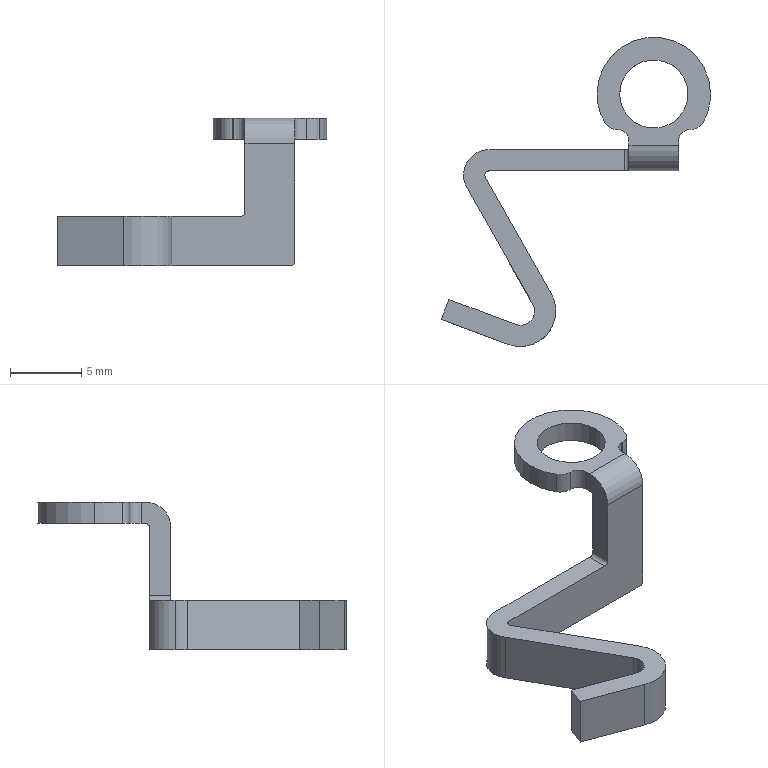Part | STEP file | TQ-DD-1105-THTerminalA1010_デフォルト | 1 solid | 34 faces | box 18.96 x 21.767 x 10.4 mm | volume 259.607 mm3 | cylinder 19 | plane 15 | commonest cylinder face diameters 0.6 x5 2 x3 3.6 x3 8 x3 1.6 x2 4.8 x2
STEP:
#1=CARTESIAN_POINT('',(-11.896,-5.7,-5.4));
#2=VERTEX_POINT('',#1);
#3=CARTESIAN_POINT('',(-11.596,-5.4,-5.4));
#4=VERTEX_POINT('',#3);
#5=CARTESIAN_POINT('',(-11.596,-5.7,-5.4));
#6=DIRECTION('',(0.,0.,-1.));
#7=DIRECTION('',(-1.,0.,0.));
#8=AXIS2_PLACEMENT_3D('',#5,#6,#7);
#9=CIRCLE('',#8,0.3);
#10=EDGE_CURVE('',#2,#4,#9,.T.);
#11=ORIENTED_EDGE('',*,*,#10,.F.);
#12=CARTESIAN_POINT('',(-11.896,-5.7,-8.9));
#13=VERTEX_POINT('',#12);
#14=CARTESIAN_POINT('',(-11.896,-5.7,-7.15));
#15=DIRECTION('',(0.,0.,-1.));
#16=VECTOR('',#15,1000.);
#17=LINE('',#14,#16);
#18=EDGE_CURVE('',#2,#13,#17,.T.);
#19=ORIENTED_EDGE('',*,*,#18,.T.);
#20=CARTESIAN_POINT('',(-11.596,-5.4,-8.9));
#21=VERTEX_POINT('',#20);
#22=CARTESIAN_POINT('',(-11.596,-5.7,-8.9));
#23=DIRECTION('',(0.,0.,1.));
#24=DIRECTION('',(-1.,0.,0.));
#25=AXIS2_PLACEMENT_3D('',#22,#23,#24);
#26=CIRCLE('',#25,0.3);
#27=EDGE_CURVE('',#21,#13,#26,.T.);
#28=ORIENTED_EDGE('',*,*,#27,.F.);
#29=CARTESIAN_POINT('',(-11.596,-5.4,0.));
#30=DIRECTION('',(0.,0.,-1.));
#31=VECTOR('',#30,1000.);
#32=LINE('',#29,#31);
#33=EDGE_CURVE('',#4,#21,#32,.T.);
#34=ORIENTED_EDGE('',*,*,#33,.F.);
#35=EDGE_LOOP('',(#11,#19,#28,#34));
#36=FACE_OUTER_BOUND('',#35,.T.);
#37=CARTESIAN_POINT('',(-11.596,-5.7,-7.15));
#38=DIRECTION('',(0.,0.,-1.));
#39=DIRECTION('',(-1.,0.,0.));
#40=AXIS2_PLACEMENT_3D('',#37,#38,#39);
#41=CYLINDRICAL_SURFACE('',#40,0.3);
#42=ADVANCED_FACE('',(#36),#41,.F.);
#43=CARTESIAN_POINT('',(-13.163,-6.586,-5.4));
#44=VERTEX_POINT('',#43);
#45=CARTESIAN_POINT('',(-13.396,-5.7,-5.4));
#46=VERTEX_POINT('',#45);
#47=CARTESIAN_POINT('',(-11.596,-5.7,-5.4));
#48=DIRECTION('',(0.,0.,-1.));
#49=DIRECTION('',(-1.,0.,0.));
#50=AXIS2_PLACEMENT_3D('',#47,#48,#49);
#51=CIRCLE('',#50,1.8);
#52=EDGE_CURVE('',#44,#46,#51,.T.);
#53=ORIENTED_EDGE('',*,*,#52,.T.);
#54=CARTESIAN_POINT('',(-13.396,-5.7,-8.9));
#55=VERTEX_POINT('',#54);
#56=CARTESIAN_POINT('',(-13.396,-5.7,-7.15));
#57=DIRECTION('',(0.,0.,-1.));
#58=VECTOR('',#57,1000.);
#59=LINE('',#56,#58);
#60=EDGE_CURVE('',#46,#55,#59,.T.);
#61=ORIENTED_EDGE('',*,*,#60,.T.);
#62=CARTESIAN_POINT('',(-13.163,-6.586,-8.9));
#63=VERTEX_POINT('',#62);
#64=CARTESIAN_POINT('',(-11.596,-5.7,-8.9));
#65=DIRECTION('',(0.,0.,-1.));
#66=DIRECTION('',(-1.,0.,0.));
#67=AXIS2_PLACEMENT_3D('',#64,#65,#66);
#68=CIRCLE('',#67,1.8);
#69=EDGE_CURVE('',#63,#55,#68,.T.);
#70=ORIENTED_EDGE('',*,*,#69,.F.);
#71=CARTESIAN_POINT('',(-13.163,-6.586,-7.15));
#72=DIRECTION('',(0.,0.,1.));
#73=VECTOR('',#72,1000.);
#74=LINE('',#71,#73);
#75=EDGE_CURVE('',#63,#44,#74,.T.);
#76=ORIENTED_EDGE('',*,*,#75,.T.);
#77=EDGE_LOOP('',(#53,#61,#70,#76));
#78=FACE_OUTER_BOUND('',#77,.T.);
#79=CARTESIAN_POINT('',(-11.596,-5.7,-7.15));
#80=DIRECTION('',(0.,0.,-1.));
#81=DIRECTION('',(-1.,0.,0.));
#82=AXIS2_PLACEMENT_3D('',#79,#80,#81);
#83=CYLINDRICAL_SURFACE('',#82,1.8);
#84=ADVANCED_FACE('',(#78),#83,.T.);
#85=CARTESIAN_POINT('',(-2.4,0.,0.));
#86=VERTEX_POINT('',#85);
#87=CARTESIAN_POINT('',(2.4,0.,0.));
#88=VERTEX_POINT('',#87);
#89=CARTESIAN_POINT('',(0.,0.,0.));
#90=DIRECTION('',(0.,0.,1.));
#91=DIRECTION('',(1.,0.,0.));
#92=AXIS2_PLACEMENT_3D('',#89,#90,#91);
#93=CIRCLE('',#92,2.4);
#94=EDGE_CURVE('',#86,#88,#93,.T.);
#95=ORIENTED_EDGE('',*,*,#94,.F.);
#96=CARTESIAN_POINT('',(-2.4,0.,1.5));
#97=VERTEX_POINT('',#96);
#98=CARTESIAN_POINT('',(-2.4,0.,0.75));
#99=DIRECTION('',(0.,0.,1.));
#100=VECTOR('',#99,1000.);
#101=LINE('',#98,#100);
#102=EDGE_CURVE('',#86,#97,#101,.T.);
#103=ORIENTED_EDGE('',*,*,#102,.T.);
#104=CARTESIAN_POINT('',(2.4,0.,1.5));
#105=VERTEX_POINT('',#104);
#106=CARTESIAN_POINT('',(0.,0.,1.5));
#107=DIRECTION('',(0.,0.,-1.));
#108=DIRECTION('',(1.,0.,0.));
#109=AXIS2_PLACEMENT_3D('',#106,#107,#108);
#110=CIRCLE('',#109,2.4);
#111=EDGE_CURVE('',#105,#97,#110,.T.);
#112=ORIENTED_EDGE('',*,*,#111,.F.);
#113=CARTESIAN_POINT('',(2.4,0.,0.75));
#114=DIRECTION('',(0.,0.,1.));
#115=VECTOR('',#114,1000.);
#116=LINE('',#113,#115);
#117=EDGE_CURVE('',#88,#105,#116,.T.);
#118=ORIENTED_EDGE('',*,*,#117,.F.);
#119=EDGE_LOOP('',(#95,#103,#112,#118));
#120=FACE_OUTER_BOUND('',#119,.T.);
#121=CARTESIAN_POINT('',(0.,0.,0.75));
#122=DIRECTION('',(0.,0.,1.));
#123=DIRECTION('',(1.,0.,0.));
#124=AXIS2_PLACEMENT_3D('',#121,#122,#123);
#125=CYLINDRICAL_SURFACE('',#124,2.4);
#126=ADVANCED_FACE('',(#120),#125,.F.);
#127=CARTESIAN_POINT('',(4.,0.,0.));
#128=VERTEX_POINT('',#127);
#129=CARTESIAN_POINT('',(-4.,0.,0.));
#130=VERTEX_POINT('',#129);
#131=CARTESIAN_POINT('',(0.,0.,0.));
#132=DIRECTION('',(0.,0.,1.));
#133=DIRECTION('',(1.,0.,0.));
#134=AXIS2_PLACEMENT_3D('',#131,#132,#133);
#135=CIRCLE('',#134,4.);
#136=EDGE_CURVE('',#128,#130,#135,.T.);
#137=ORIENTED_EDGE('',*,*,#136,.T.);
#138=CARTESIAN_POINT('',(-4.,0.,1.5));
#139=VERTEX_POINT('',#138);
#140=CARTESIAN_POINT('',(-4.,0.,0.75));
#141=DIRECTION('',(0.,0.,1.));
#142=VECTOR('',#141,1000.);
#143=LINE('',#140,#142);
#144=EDGE_CURVE('',#130,#139,#143,.T.);
#145=ORIENTED_EDGE('',*,*,#144,.T.);
#146=CARTESIAN_POINT('',(4.,0.,1.5));
#147=VERTEX_POINT('',#146);
#148=CARTESIAN_POINT('',(0.,0.,1.5));
#149=DIRECTION('',(0.,0.,1.));
#150=DIRECTION('',(1.,0.,0.));
#151=AXIS2_PLACEMENT_3D('',#148,#149,#150);
#152=CIRCLE('',#151,4.);
#153=EDGE_CURVE('',#147,#139,#152,.T.);
#154=ORIENTED_EDGE('',*,*,#153,.F.);
#155=CARTESIAN_POINT('',(4.,0.,0.75));
#156=DIRECTION('',(0.,0.,1.));
#157=VECTOR('',#156,1000.);
#158=LINE('',#155,#157);
#159=EDGE_CURVE('',#128,#147,#158,.T.);
#160=ORIENTED_EDGE('',*,*,#159,.F.);
#161=EDGE_LOOP('',(#137,#145,#154,#160));
#162=FACE_OUTER_BOUND('',#161,.T.);
#163=CARTESIAN_POINT('',(0.,0.,0.75));
#164=DIRECTION('',(0.,0.,1.));
#165=DIRECTION('',(1.,0.,0.));
#166=AXIS2_PLACEMENT_3D('',#163,#164,#165);
#167=CYLINDRICAL_SURFACE('',#166,4.);
#168=ADVANCED_FACE('',(#162),#167,.T.);
#169=CARTESIAN_POINT('',(3.464,-2.,0.));
#170=VERTEX_POINT('',#169);
#171=CARTESIAN_POINT('',(0.,0.,0.));
#172=DIRECTION('',(0.,0.,1.));
#173=DIRECTION('',(1.,0.,0.));
#174=AXIS2_PLACEMENT_3D('',#171,#172,#173);
#175=CIRCLE('',#174,4.);
#176=EDGE_CURVE('',#170,#128,#175,.T.);
#177=ORIENTED_EDGE('',*,*,#176,.T.);
#178=ORIENTED_EDGE('',*,*,#159,.T.);
#179=CARTESIAN_POINT('',(3.464,-2.,1.5));
#180=VERTEX_POINT('',#179);
#181=CARTESIAN_POINT('',(0.,0.,1.5));
#182=DIRECTION('',(0.,0.,1.));
#183=DIRECTION('',(1.,0.,0.));
#184=AXIS2_PLACEMENT_3D('',#181,#182,#183);
#185=CIRCLE('',#184,4.);
#186=EDGE_CURVE('',#180,#147,#185,.T.);
#187=ORIENTED_EDGE('',*,*,#186,.F.);
#188=CARTESIAN_POINT('',(3.464,-2.,0.75));
#189=DIRECTION('',(0.,0.,1.));
#190=VECTOR('',#189,1000.);
#191=LINE('',#188,#190);
#192=EDGE_CURVE('',#170,#180,#191,.T.);
#193=ORIENTED_EDGE('',*,*,#192,.F.);
#194=EDGE_LOOP('',(#177,#178,#187,#193));
#195=FACE_OUTER_BOUND('',#194,.T.);
#196=CARTESIAN_POINT('',(0.,0.,0.75));
#197=DIRECTION('',(0.,0.,1.));
#198=DIRECTION('',(1.,0.,0.));
#199=AXIS2_PLACEMENT_3D('',#196,#197,#198);
#200=CYLINDRICAL_SURFACE('',#199,4.);
#201=ADVANCED_FACE('',(#195),#200,.T.);
#202=CARTESIAN_POINT('',(1.75,-5.4,-0.3));
#203=VERTEX_POINT('',#202);
#204=CARTESIAN_POINT('',(-1.75,-5.4,-0.3));
#205=VERTEX_POINT('',#204);
#206=CARTESIAN_POINT('',(-1.75,-5.4,-0.3));
#207=DIRECTION('',(-1.,0.,0.));
#208=VECTOR('',#207,1000.);
#209=LINE('',#206,#208);
#210=EDGE_CURVE('',#203,#205,#209,.T.);
#211=ORIENTED_EDGE('',*,*,#210,.T.);
#212=CARTESIAN_POINT('',(-1.75,-5.4,-5.1));
#213=VERTEX_POINT('',#212);
#214=CARTESIAN_POINT('',(-1.75,-5.4,0.));
#215=DIRECTION('',(0.,0.,-1.));
#216=VECTOR('',#215,1000.);
#217=LINE('',#214,#216);
#218=EDGE_CURVE('',#205,#213,#217,.T.);
#219=ORIENTED_EDGE('',*,*,#218,.T.);
#220=CARTESIAN_POINT('',(-2.05,-5.4,-5.4));
#221=VERTEX_POINT('',#220);
#222=CARTESIAN_POINT('',(-2.05,-5.4,-5.1));
#223=DIRECTION('',(0.,1.,0.));
#224=DIRECTION('',(0.,0.,1.));
#225=AXIS2_PLACEMENT_3D('',#222,#223,#224);
#226=CIRCLE('',#225,0.3);
#227=EDGE_CURVE('',#213,#221,#226,.T.);
#228=ORIENTED_EDGE('',*,*,#227,.T.);
#229=CARTESIAN_POINT('',(-1.75,-5.4,-5.4));
#230=DIRECTION('',(-1.,0.,0.));
#231=VECTOR('',#230,1000.);
#232=LINE('',#229,#231);
#233=EDGE_CURVE('',#221,#4,#232,.T.);
#234=ORIENTED_EDGE('',*,*,#233,.T.);
#235=ORIENTED_EDGE('',*,*,#33,.T.);
#236=CARTESIAN_POINT('',(1.45,-5.4,-8.9));
#237=VERTEX_POINT('',#236);
#238=CARTESIAN_POINT('',(-1.75,-5.4,-8.9));
#239=DIRECTION('',(1.,0.,0.));
#240=VECTOR('',#239,1000.);
#241=LINE('',#238,#240);
#242=EDGE_CURVE('',#21,#237,#241,.T.);
#243=ORIENTED_EDGE('',*,*,#242,.T.);
#244=CARTESIAN_POINT('',(1.75,-5.4,-8.6));
#245=VERTEX_POINT('',#244);
#246=CARTESIAN_POINT('',(1.45,-5.4,-8.6));
#247=DIRECTION('',(0.,1.,0.));
#248=DIRECTION('',(0.,0.,1.));
#249=AXIS2_PLACEMENT_3D('',#246,#247,#248);
#250=CIRCLE('',#249,0.3);
#251=EDGE_CURVE('',#245,#237,#250,.T.);
#252=ORIENTED_EDGE('',*,*,#251,.F.);
#253=CARTESIAN_POINT('',(1.75,-5.4,0.));
#254=DIRECTION('',(0.,0.,1.));
#255=VECTOR('',#254,1000.);
#256=LINE('',#253,#255);
#257=EDGE_CURVE('',#245,#203,#256,.T.);
#258=ORIENTED_EDGE('',*,*,#257,.T.);
#259=EDGE_LOOP('',(#211,#219,#228,#234,#235,#243,#252,#258));
#260=FACE_OUTER_BOUND('',#259,.T.);
#261=CARTESIAN_POINT('',(-1.75,-5.4,0.));
#262=DIRECTION('',(0.,-1.,0.));
#263=DIRECTION('',(0.,0.,-1.));
#264=AXIS2_PLACEMENT_3D('',#261,#262,#263);
#265=PLANE('',#264);
#266=ADVANCED_FACE('',(#260),#265,.T.);
#267=CARTESIAN_POINT('',(-1.75,-3.9,-0.3));
#268=VERTEX_POINT('',#267);
#269=CARTESIAN_POINT('',(-1.75,-3.9,-5.1));
#270=VERTEX_POINT('',#269);
#271=CARTESIAN_POINT('',(-1.75,-3.9,0.));
#272=DIRECTION('',(0.,0.,-1.));
#273=VECTOR('',#272,1000.);
#274=LINE('',#271,#273);
#275=EDGE_CURVE('',#268,#270,#274,.T.);
#276=ORIENTED_EDGE('',*,*,#275,.T.);
#277=CARTESIAN_POINT('',(-1.75,-2.5,-5.1));
#278=DIRECTION('',(0.,-1.,0.));
#279=VECTOR('',#278,1000.);
#280=LINE('',#277,#279);
#281=EDGE_CURVE('',#270,#213,#280,.T.);
#282=ORIENTED_EDGE('',*,*,#281,.T.);
#283=ORIENTED_EDGE('',*,*,#218,.F.);
#284=CARTESIAN_POINT('',(-1.75,-3.6,1.5));
#285=VERTEX_POINT('',#284);
#286=CARTESIAN_POINT('',(-1.75,-3.6,-0.3));
#287=DIRECTION('',(-1.,0.,0.));
#288=DIRECTION('',(0.,0.,-1.));
#289=AXIS2_PLACEMENT_3D('',#286,#287,#288);
#290=CIRCLE('',#289,1.8);
#291=EDGE_CURVE('',#205,#285,#290,.T.);
#292=ORIENTED_EDGE('',*,*,#291,.T.);
#293=CARTESIAN_POINT('',(-1.75,-3.3,1.5));
#294=VERTEX_POINT('',#293);
#295=CARTESIAN_POINT('',(-1.75,0.,1.5));
#296=DIRECTION('',(0.,-1.,0.));
#297=VECTOR('',#296,1000.);
#298=LINE('',#295,#297);
#299=EDGE_CURVE('',#294,#285,#298,.T.);
#300=ORIENTED_EDGE('',*,*,#299,.F.);
#301=CARTESIAN_POINT('',(-1.75,-3.3,0.));
#302=VERTEX_POINT('',#301);
#303=CARTESIAN_POINT('',(-1.75,-3.3,0.));
#304=DIRECTION('',(0.,0.,-1.));
#305=VECTOR('',#304,1000.);
#306=LINE('',#303,#305);
#307=EDGE_CURVE('',#294,#302,#306,.T.);
#308=ORIENTED_EDGE('',*,*,#307,.T.);
#309=CARTESIAN_POINT('',(-1.75,-3.6,0.));
#310=VERTEX_POINT('',#309);
#311=CARTESIAN_POINT('',(-1.75,0.,0.));
#312=DIRECTION('',(0.,-1.,0.));
#313=VECTOR('',#312,1000.);
#314=LINE('',#311,#313);
#315=EDGE_CURVE('',#302,#310,#314,.T.);
#316=ORIENTED_EDGE('',*,*,#315,.T.);
#317=CARTESIAN_POINT('',(-1.75,-3.6,-0.3));
#318=DIRECTION('',(1.,0.,0.));
#319=DIRECTION('',(0.,0.,1.));
#320=AXIS2_PLACEMENT_3D('',#317,#318,#319);
#321=CIRCLE('',#320,0.3);
#322=EDGE_CURVE('',#310,#268,#321,.T.);
#323=ORIENTED_EDGE('',*,*,#322,.T.);
#324=EDGE_LOOP('',(#276,#282,#283,#292,#300,#308,#316,#323));
#325=FACE_OUTER_BOUND('',#324,.T.);
#326=CARTESIAN_POINT('',(-1.75,-2.5,0.));
#327=DIRECTION('',(-1.,0.,0.));
#328=DIRECTION('',(0.,0.,1.));
#329=AXIS2_PLACEMENT_3D('',#326,#327,#328);
#330=PLANE('',#329);
#331=ADVANCED_FACE('',(#325),#330,.T.);
#332=ORIENTED_EDGE('',*,*,#291,.F.);
#333=ORIENTED_EDGE('',*,*,#210,.F.);
#334=CARTESIAN_POINT('',(1.75,-3.6,1.5));
#335=VERTEX_POINT('',#334);
#336=CARTESIAN_POINT('',(1.75,-3.6,-0.3));
#337=DIRECTION('',(-1.,0.,0.));
#338=DIRECTION('',(0.,0.,-1.));
#339=AXIS2_PLACEMENT_3D('',#336,#337,#338);
#340=CIRCLE('',#339,1.8);
#341=EDGE_CURVE('',#203,#335,#340,.T.);
#342=ORIENTED_EDGE('',*,*,#341,.T.);
#343=CARTESIAN_POINT('',(0.,-3.6,1.5));
#344=DIRECTION('',(-1.,0.,0.));
#345=VECTOR('',#344,1000.);
#346=LINE('',#343,#345);
#347=EDGE_CURVE('',#335,#285,#346,.T.);
#348=ORIENTED_EDGE('',*,*,#347,.T.);
#349=EDGE_LOOP('',(#332,#333,#342,#348));
#350=FACE_OUTER_BOUND('',#349,.T.);
#351=CARTESIAN_POINT('',(0.,-3.6,-0.3));
#352=DIRECTION('',(1.,0.,0.));
#353=DIRECTION('',(0.,0.,-1.));
#354=AXIS2_PLACEMENT_3D('',#351,#352,#353);
#355=CYLINDRICAL_SURFACE('',#354,1.8);
#356=ADVANCED_FACE('',(#350),#355,.T.);
#357=ORIENTED_EDGE('',*,*,#257,.F.);
#358=CARTESIAN_POINT('',(1.75,-3.9,-8.6));
#359=VERTEX_POINT('',#358);
#360=CARTESIAN_POINT('',(1.75,-5.4,-8.6));
#361=DIRECTION('',(0.,1.,0.));
#362=VECTOR('',#361,1000.);
#363=LINE('',#360,#362);
#364=EDGE_CURVE('',#245,#359,#363,.T.);
#365=ORIENTED_EDGE('',*,*,#364,.T.);
#366=CARTESIAN_POINT('',(1.75,-3.9,-0.3));
#367=VERTEX_POINT('',#366);
#368=CARTESIAN_POINT('',(1.75,-3.9,0.));
#369=DIRECTION('',(0.,0.,1.));
#370=VECTOR('',#369,1000.);
#371=LINE('',#368,#370);
#372=EDGE_CURVE('',#359,#367,#371,.T.);
#373=ORIENTED_EDGE('',*,*,#372,.T.);
#374=CARTESIAN_POINT('',(1.75,-3.6,0.));
#375=VERTEX_POINT('',#374);
#376=CARTESIAN_POINT('',(1.75,-3.6,-0.3));
#377=DIRECTION('',(-1.,0.,0.));
#378=DIRECTION('',(0.,0.,1.));
#379=AXIS2_PLACEMENT_3D('',#376,#377,#378);
#380=CIRCLE('',#379,0.3);
#381=EDGE_CURVE('',#367,#375,#380,.T.);
#382=ORIENTED_EDGE('',*,*,#381,.T.);
#383=CARTESIAN_POINT('',(1.75,-3.3,0.));
#384=VERTEX_POINT('',#383);
#385=CARTESIAN_POINT('',(1.75,0.,0.));
#386=DIRECTION('',(0.,1.,0.));
#387=VECTOR('',#386,1000.);
#388=LINE('',#385,#387);
#389=EDGE_CURVE('',#375,#384,#388,.T.);
#390=ORIENTED_EDGE('',*,*,#389,.T.);
#391=CARTESIAN_POINT('',(1.75,-3.3,1.5));
#392=VERTEX_POINT('',#391);
#393=CARTESIAN_POINT('',(1.75,-3.3,0.));
#394=DIRECTION('',(0.,0.,1.));
#395=VECTOR('',#394,1000.);
#396=LINE('',#393,#395);
#397=EDGE_CURVE('',#384,#392,#396,.T.);
#398=ORIENTED_EDGE('',*,*,#397,.T.);
#399=CARTESIAN_POINT('',(1.75,-5.4,1.5));
#400=DIRECTION('',(0.,-1.,0.));
#401=VECTOR('',#400,1000.);
#402=LINE('',#399,#401);
#403=EDGE_CURVE('',#392,#335,#402,.T.);
#404=ORIENTED_EDGE('',*,*,#403,.T.);
#405=ORIENTED_EDGE('',*,*,#341,.F.);
#406=EDGE_LOOP('',(#357,#365,#373,#382,#390,#398,#404,#405));
#407=FACE_OUTER_BOUND('',#406,.T.);
#408=CARTESIAN_POINT('',(1.75,-5.4,0.));
#409=DIRECTION('',(1.,0.,0.));
#410=DIRECTION('',(0.,0.,-1.));
#411=AXIS2_PLACEMENT_3D('',#408,#409,#410);
#412=PLANE('',#411);
#413=ADVANCED_FACE('',(#407),#412,.T.);
#414=CARTESIAN_POINT('',(-11.596,-3.9,-8.9));
#415=VERTEX_POINT('',#414);
#416=CARTESIAN_POINT('',(1.45,-3.9,-8.9));
#417=VERTEX_POINT('',#416);
#418=CARTESIAN_POINT('',(0.,-3.9,-8.9));
#419=DIRECTION('',(1.,0.,0.));
#420=VECTOR('',#419,1000.);
#421=LINE('',#418,#420);
#422=EDGE_CURVE('',#415,#417,#421,.T.);
#423=ORIENTED_EDGE('',*,*,#422,.T.);
#424=CARTESIAN_POINT('',(1.45,-5.4,-8.9));
#425=DIRECTION('',(0.,-1.,0.));
#426=VECTOR('',#425,1000.);
#427=LINE('',#424,#426);
#428=EDGE_CURVE('',#417,#237,#427,.T.);
#429=ORIENTED_EDGE('',*,*,#428,.T.);
#430=ORIENTED_EDGE('',*,*,#242,.F.);
#431=ORIENTED_EDGE('',*,*,#27,.T.);
#432=CARTESIAN_POINT('',(-11.857,-5.848,-8.9));
#433=VERTEX_POINT('',#432);
#434=CARTESIAN_POINT('',(-11.596,-5.7,-8.9));
#435=DIRECTION('',(0.,0.,1.));
#436=DIRECTION('',(-1.,0.,0.));
#437=AXIS2_PLACEMENT_3D('',#434,#435,#436);
#438=CIRCLE('',#437,0.3);
#439=EDGE_CURVE('',#13,#433,#438,.T.);
#440=ORIENTED_EDGE('',*,*,#439,.T.);
#441=CARTESIAN_POINT('',(-7.225,-14.036,-8.9));
#442=VERTEX_POINT('',#441);
#443=CARTESIAN_POINT('',(-11.857,-5.848,-8.9));
#444=DIRECTION('',(0.4924,-0.8704,0.));
#445=VECTOR('',#444,1000.);
#446=LINE('',#443,#445);
#447=EDGE_CURVE('',#433,#442,#446,.T.);
#448=ORIENTED_EDGE('',*,*,#447,.T.);
#449=CARTESIAN_POINT('',(-10.276,-17.608,-8.9));
#450=VERTEX_POINT('',#449);
#451=CARTESIAN_POINT('',(-9.401,-15.267,-8.9));
#452=DIRECTION('',(0.,0.,-1.));
#453=DIRECTION('',(-1.,0.,0.));
#454=AXIS2_PLACEMENT_3D('',#451,#452,#453);
#455=CIRCLE('',#454,2.5);
#456=EDGE_CURVE('',#442,#450,#455,.T.);
#457=ORIENTED_EDGE('',*,*,#456,.T.);
#458=CARTESIAN_POINT('',(-14.96,-15.857,-8.9));
#459=VERTEX_POINT('',#458);
#460=CARTESIAN_POINT('',(-10.276,-17.608,-8.9));
#461=DIRECTION('',(-0.9367,0.3502,0.));
#462=VECTOR('',#461,1000.);
#463=LINE('',#460,#462);
#464=EDGE_CURVE('',#450,#459,#463,.T.);
#465=ORIENTED_EDGE('',*,*,#464,.T.);
#466=CARTESIAN_POINT('',(-14.434,-14.452,-8.9));
#467=VERTEX_POINT('',#466);
#468=CARTESIAN_POINT('',(-14.434,-14.452,-8.9));
#469=DIRECTION('',(-0.3502,-0.9367,0.));
#470=VECTOR('',#469,1000.);
#471=LINE('',#468,#470);
#472=EDGE_CURVE('',#467,#459,#471,.T.);
#473=ORIENTED_EDGE('',*,*,#472,.F.);
#474=CARTESIAN_POINT('',(-9.751,-16.203,-8.9));
#475=VERTEX_POINT('',#474);
#476=CARTESIAN_POINT('',(-14.434,-14.452,-8.9));
#477=DIRECTION('',(0.9367,-0.3502,0.));
#478=VECTOR('',#477,1000.);
#479=LINE('',#476,#478);
#480=EDGE_CURVE('',#467,#475,#479,.T.);
#481=ORIENTED_EDGE('',*,*,#480,.T.);
#482=CARTESIAN_POINT('',(-8.53,-14.774,-8.9));
#483=VERTEX_POINT('',#482);
#484=CARTESIAN_POINT('',(-9.401,-15.267,-8.9));
#485=DIRECTION('',(0.,0.,1.));
#486=DIRECTION('',(-1.,0.,0.));
#487=AXIS2_PLACEMENT_3D('',#484,#485,#486);
#488=CIRCLE('',#487,1.);
#489=EDGE_CURVE('',#475,#483,#488,.T.);
#490=ORIENTED_EDGE('',*,*,#489,.T.);
#491=CARTESIAN_POINT('',(-8.53,-14.774,-8.9));
#492=DIRECTION('',(-0.4924,0.8704,0.));
#493=VECTOR('',#492,1000.);
#494=LINE('',#491,#493);
#495=EDGE_CURVE('',#483,#63,#494,.T.);
#496=ORIENTED_EDGE('',*,*,#495,.T.);
#497=ORIENTED_EDGE('',*,*,#69,.T.);
#498=CARTESIAN_POINT('',(-11.596,-5.7,-8.9));
#499=DIRECTION('',(0.,0.,-1.));
#500=DIRECTION('',(-1.,0.,0.));
#501=AXIS2_PLACEMENT_3D('',#498,#499,#500);
#502=CIRCLE('',#501,1.8);
#503=EDGE_CURVE('',#55,#415,#502,.T.);
#504=ORIENTED_EDGE('',*,*,#503,.T.);
#505=EDGE_LOOP('',(#423,#429,#430,#431,#440,#448,#457,#465,#473,#481,#490,#496,#497,#504));
#506=FACE_OUTER_BOUND('',#505,.T.);
#507=CARTESIAN_POINT('',(0.,-5.4,-8.9));
#508=DIRECTION('',(0.,0.,-1.));
#509=DIRECTION('',(-1.,0.,0.));
#510=AXIS2_PLACEMENT_3D('',#507,#508,#509);
#511=PLANE('',#510);
#512=ADVANCED_FACE('',(#506),#511,.T.);
#513=ORIENTED_EDGE('',*,*,#18,.F.);
#514=CARTESIAN_POINT('',(-11.857,-5.848,-5.4));
#515=VERTEX_POINT('',#514);
#516=CARTESIAN_POINT('',(-11.596,-5.7,-5.4));
#517=DIRECTION('',(0.,0.,-1.));
#518=DIRECTION('',(-1.,0.,0.));
#519=AXIS2_PLACEMENT_3D('',#516,#517,#518);
#520=CIRCLE('',#519,0.3);
#521=EDGE_CURVE('',#515,#2,#520,.T.);
#522=ORIENTED_EDGE('',*,*,#521,.F.);
#523=CARTESIAN_POINT('',(-11.857,-5.848,-7.15));
#524=DIRECTION('',(0.,0.,1.));
#525=VECTOR('',#524,1000.);
#526=LINE('',#523,#525);
#527=EDGE_CURVE('',#433,#515,#526,.T.);
#528=ORIENTED_EDGE('',*,*,#527,.F.);
#529=ORIENTED_EDGE('',*,*,#439,.F.);
#530=EDGE_LOOP('',(#513,#522,#528,#529));
#531=FACE_OUTER_BOUND('',#530,.T.);
#532=CARTESIAN_POINT('',(-11.596,-5.7,-7.15));
#533=DIRECTION('',(0.,0.,-1.));
#534=DIRECTION('',(-1.,0.,0.));
#535=AXIS2_PLACEMENT_3D('',#532,#533,#534);
#536=CYLINDRICAL_SURFACE('',#535,0.3);
#537=ADVANCED_FACE('',(#531),#536,.F.);
#538=CARTESIAN_POINT('',(-11.596,-3.9,-5.4));
#539=VERTEX_POINT('',#538);
#540=CARTESIAN_POINT('',(-2.05,-3.9,-5.4));
#541=VERTEX_POINT('',#540);
#542=CARTESIAN_POINT('',(0.,-3.9,-5.4));
#543=DIRECTION('',(1.,0.,0.));
#544=VECTOR('',#543,1000.);
#545=LINE('',#542,#544);
#546=EDGE_CURVE('',#539,#541,#545,.T.);
#547=ORIENTED_EDGE('',*,*,#546,.F.);
#548=CARTESIAN_POINT('',(-11.596,-5.7,-5.4));
#549=DIRECTION('',(0.,0.,-1.));
#550=DIRECTION('',(-1.,0.,0.));
#551=AXIS2_PLACEMENT_3D('',#548,#549,#550);
#552=CIRCLE('',#551,1.8);
#553=EDGE_CURVE('',#46,#539,#552,.T.);
#554=ORIENTED_EDGE('',*,*,#553,.F.);
#555=ORIENTED_EDGE('',*,*,#52,.F.);
#556=CARTESIAN_POINT('',(-8.53,-14.774,-5.4));
#557=VERTEX_POINT('',#556);
#558=CARTESIAN_POINT('',(-8.53,-14.774,-5.4));
#559=DIRECTION('',(-0.4924,0.8704,0.));
#560=VECTOR('',#559,1000.);
#561=LINE('',#558,#560);
#562=EDGE_CURVE('',#557,#44,#561,.T.);
#563=ORIENTED_EDGE('',*,*,#562,.F.);
#564=CARTESIAN_POINT('',(-9.751,-16.203,-5.4));
#565=VERTEX_POINT('',#564);
#566=CARTESIAN_POINT('',(-9.401,-15.267,-5.4));
#567=DIRECTION('',(0.,0.,1.));
#568=DIRECTION('',(-1.,0.,0.));
#569=AXIS2_PLACEMENT_3D('',#566,#567,#568);
#570=CIRCLE('',#569,1.);
#571=EDGE_CURVE('',#565,#557,#570,.T.);
#572=ORIENTED_EDGE('',*,*,#571,.F.);
#573=CARTESIAN_POINT('',(-14.434,-14.452,-5.4));
#574=VERTEX_POINT('',#573);
#575=CARTESIAN_POINT('',(-14.434,-14.452,-5.4));
#576=DIRECTION('',(0.9367,-0.3502,0.));
#577=VECTOR('',#576,1000.);
#578=LINE('',#575,#577);
#579=EDGE_CURVE('',#574,#565,#578,.T.);
#580=ORIENTED_EDGE('',*,*,#579,.F.);
#581=CARTESIAN_POINT('',(-14.96,-15.857,-5.4));
#582=VERTEX_POINT('',#581);
#583=CARTESIAN_POINT('',(-14.434,-14.452,-5.4));
#584=DIRECTION('',(0.3502,0.9367,0.));
#585=VECTOR('',#584,1000.);
#586=LINE('',#583,#585);
#587=EDGE_CURVE('',#582,#574,#586,.T.);
#588=ORIENTED_EDGE('',*,*,#587,.F.);
#589=CARTESIAN_POINT('',(-10.276,-17.608,-5.4));
#590=VERTEX_POINT('',#589);
#591=CARTESIAN_POINT('',(-10.276,-17.608,-5.4));
#592=DIRECTION('',(-0.9367,0.3502,0.));
#593=VECTOR('',#592,1000.);
#594=LINE('',#591,#593);
#595=EDGE_CURVE('',#590,#582,#594,.T.);
#596=ORIENTED_EDGE('',*,*,#595,.F.);
#597=CARTESIAN_POINT('',(-7.225,-14.036,-5.4));
#598=VERTEX_POINT('',#597);
#599=CARTESIAN_POINT('',(-9.401,-15.267,-5.4));
#600=DIRECTION('',(0.,0.,-1.));
#601=DIRECTION('',(-1.,0.,0.));
#602=AXIS2_PLACEMENT_3D('',#599,#600,#601);
#603=CIRCLE('',#602,2.5);
#604=EDGE_CURVE('',#598,#590,#603,.T.);
#605=ORIENTED_EDGE('',*,*,#604,.F.);
#606=CARTESIAN_POINT('',(-11.857,-5.848,-5.4));
#607=DIRECTION('',(0.4924,-0.8704,0.));
#608=VECTOR('',#607,1000.);
#609=LINE('',#606,#608);
#610=EDGE_CURVE('',#515,#598,#609,.T.);
#611=ORIENTED_EDGE('',*,*,#610,.F.);
#612=ORIENTED_EDGE('',*,*,#521,.T.);
#613=ORIENTED_EDGE('',*,*,#10,.T.);
#614=ORIENTED_EDGE('',*,*,#233,.F.);
#615=CARTESIAN_POINT('',(-2.05,0.,-5.4));
#616=DIRECTION('',(0.,-1.,0.));
#617=VECTOR('',#616,1000.);
#618=LINE('',#615,#617);
#619=EDGE_CURVE('',#541,#221,#618,.T.);
#620=ORIENTED_EDGE('',*,*,#619,.F.);
#621=EDGE_LOOP('',(#547,#554,#555,#563,#572,#580,#588,#596,#605,#611,#612,#613,#614,#620));
#622=FACE_OUTER_BOUND('',#621,.T.);
#623=CARTESIAN_POINT('',(0.,0.,-5.4));
#624=DIRECTION('',(0.,0.,-1.));
#625=DIRECTION('',(-1.,0.,0.));
#626=AXIS2_PLACEMENT_3D('',#623,#624,#625);
#627=PLANE('',#626);
#628=ADVANCED_FACE('',(#622),#627,.F.);
#629=CARTESIAN_POINT('',(-2.05,-3.9,-5.1));
#630=DIRECTION('',(0.,-1.,0.));
#631=DIRECTION('',(0.,0.,1.));
#632=AXIS2_PLACEMENT_3D('',#629,#630,#631);
#633=CIRCLE('',#632,0.3);
#634=EDGE_CURVE('',#541,#270,#633,.T.);
#635=ORIENTED_EDGE('',*,*,#634,.F.);
#636=ORIENTED_EDGE('',*,*,#619,.T.);
#637=ORIENTED_EDGE('',*,*,#227,.F.);
#638=ORIENTED_EDGE('',*,*,#281,.F.);
#639=EDGE_LOOP('',(#635,#636,#637,#638));
#640=FACE_OUTER_BOUND('',#639,.T.);
#641=CARTESIAN_POINT('',(-2.05,-10.833,-5.1));
#642=DIRECTION('',(0.,1.,0.));
#643=DIRECTION('',(0.,0.,1.));
#644=AXIS2_PLACEMENT_3D('',#641,#642,#643);
#645=CYLINDRICAL_SURFACE('',#644,0.3);
#646=ADVANCED_FACE('',(#640),#645,.F.);
#647=CARTESIAN_POINT('',(0.,-3.9,-0.3));
#648=DIRECTION('',(-1.,0.,0.));
#649=VECTOR('',#648,1000.);
#650=LINE('',#647,#649);
#651=EDGE_CURVE('',#367,#268,#650,.T.);
#652=ORIENTED_EDGE('',*,*,#651,.F.);
#653=ORIENTED_EDGE('',*,*,#372,.F.);
#654=CARTESIAN_POINT('',(1.45,-3.9,-8.6));
#655=DIRECTION('',(0.,-1.,0.));
#656=DIRECTION('',(0.,0.,1.));
#657=AXIS2_PLACEMENT_3D('',#654,#655,#656);
#658=CIRCLE('',#657,0.3);
#659=EDGE_CURVE('',#417,#359,#658,.T.);
#660=ORIENTED_EDGE('',*,*,#659,.F.);
#661=ORIENTED_EDGE('',*,*,#422,.F.);
#662=CARTESIAN_POINT('',(-11.596,-3.9,1.5));
#663=DIRECTION('',(0.,0.,-1.));
#664=VECTOR('',#663,1000.);
#665=LINE('',#662,#664);
#666=EDGE_CURVE('',#539,#415,#665,.T.);
#667=ORIENTED_EDGE('',*,*,#666,.F.);
#668=ORIENTED_EDGE('',*,*,#546,.T.);
#669=ORIENTED_EDGE('',*,*,#634,.T.);
#670=ORIENTED_EDGE('',*,*,#275,.F.);
#671=EDGE_LOOP('',(#652,#653,#660,#661,#667,#668,#669,#670));
#672=FACE_OUTER_BOUND('',#671,.T.);
#673=CARTESIAN_POINT('',(0.,-3.9,1.5));
#674=DIRECTION('',(0.,-1.,0.));
#675=DIRECTION('',(0.,0.,-1.));
#676=AXIS2_PLACEMENT_3D('',#673,#674,#675);
#677=PLANE('',#676);
#678=ADVANCED_FACE('',(#672),#677,.F.);
#679=CARTESIAN_POINT('',(-2.55,-2.5,1.5));
#680=VERTEX_POINT('',#679);
#681=CARTESIAN_POINT('',(-2.55,-3.3,1.5));
#682=DIRECTION('',(0.,0.,-1.));
#683=DIRECTION('',(1.,0.,0.));
#684=AXIS2_PLACEMENT_3D('',#681,#682,#683);
#685=CIRCLE('',#684,0.8);
#686=EDGE_CURVE('',#680,#294,#685,.T.);
#687=ORIENTED_EDGE('',*,*,#686,.F.);
#688=CARTESIAN_POINT('',(-2.55,-2.5,0.));
#689=VERTEX_POINT('',#688);
#690=CARTESIAN_POINT('',(-2.55,-2.5,-3.7));
#691=DIRECTION('',(0.,0.,1.));
#692=VECTOR('',#691,1000.);
#693=LINE('',#690,#692);
#694=EDGE_CURVE('',#689,#680,#693,.T.);
#695=ORIENTED_EDGE('',*,*,#694,.F.);
#696=CARTESIAN_POINT('',(-2.55,-3.3,0.));
#697=DIRECTION('',(0.,0.,-1.));
#698=DIRECTION('',(1.,0.,0.));
#699=AXIS2_PLACEMENT_3D('',#696,#697,#698);
#700=CIRCLE('',#699,0.8);
#701=EDGE_CURVE('',#689,#302,#700,.T.);
#702=ORIENTED_EDGE('',*,*,#701,.T.);
#703=ORIENTED_EDGE('',*,*,#307,.F.);
#704=EDGE_LOOP('',(#687,#695,#702,#703));
#705=FACE_OUTER_BOUND('',#704,.T.);
#706=CARTESIAN_POINT('',(-2.55,-3.3,-3.7));
#707=DIRECTION('',(0.,0.,1.));
#708=DIRECTION('',(1.,0.,0.));
#709=AXIS2_PLACEMENT_3D('',#706,#707,#708);
#710=CYLINDRICAL_SURFACE('',#709,0.8);
#711=ADVANCED_FACE('',(#705),#710,.F.);
#712=ORIENTED_EDGE('',*,*,#111,.T.);
#713=CARTESIAN_POINT('',(0.,0.,1.5));
#714=DIRECTION('',(0.,0.,-1.));
#715=DIRECTION('',(1.,0.,0.));
#716=AXIS2_PLACEMENT_3D('',#713,#714,#715);
#717=CIRCLE('',#716,2.4);
#718=EDGE_CURVE('',#97,#105,#717,.T.);
#719=ORIENTED_EDGE('',*,*,#718,.T.);
#720=EDGE_LOOP('',(#712,#719));
#721=FACE_BOUND('',#720,.T.);
#722=CARTESIAN_POINT('',(2.55,-2.5,1.5));
#723=VERTEX_POINT('',#722);
#724=CARTESIAN_POINT('',(2.598,-2.5,1.5));
#725=VERTEX_POINT('',#724);
#726=CARTESIAN_POINT('',(-1.75,-2.5,1.5));
#727=DIRECTION('',(1.,0.,0.));
#728=VECTOR('',#727,1000.);
#729=LINE('',#726,#728);
#730=EDGE_CURVE('',#723,#725,#729,.T.);
#731=ORIENTED_EDGE('',*,*,#730,.T.);
#732=CARTESIAN_POINT('',(2.598,-1.5,1.5));
#733=DIRECTION('',(0.,0.,1.));
#734=DIRECTION('',(1.,0.,0.));
#735=AXIS2_PLACEMENT_3D('',#732,#733,#734);
#736=CIRCLE('',#735,1.);
#737=EDGE_CURVE('',#725,#180,#736,.T.);
#738=ORIENTED_EDGE('',*,*,#737,.T.);
#739=ORIENTED_EDGE('',*,*,#186,.T.);
#740=ORIENTED_EDGE('',*,*,#153,.T.);
#741=CARTESIAN_POINT('',(-3.464,-2.,1.5));
#742=VERTEX_POINT('',#741);
#743=CARTESIAN_POINT('',(0.,0.,1.5));
#744=DIRECTION('',(0.,0.,1.));
#745=DIRECTION('',(1.,0.,0.));
#746=AXIS2_PLACEMENT_3D('',#743,#744,#745);
#747=CIRCLE('',#746,4.);
#748=EDGE_CURVE('',#139,#742,#747,.T.);
#749=ORIENTED_EDGE('',*,*,#748,.T.);
#750=CARTESIAN_POINT('',(-2.598,-2.5,1.5));
#751=VERTEX_POINT('',#750);
#752=CARTESIAN_POINT('',(-2.598,-1.5,1.5));
#753=DIRECTION('',(0.,0.,1.));
#754=DIRECTION('',(1.,0.,0.));
#755=AXIS2_PLACEMENT_3D('',#752,#753,#754);
#756=CIRCLE('',#755,1.);
#757=EDGE_CURVE('',#742,#751,#756,.T.);
#758=ORIENTED_EDGE('',*,*,#757,.T.);
#759=CARTESIAN_POINT('',(0.,-2.5,1.5));
#760=DIRECTION('',(1.,0.,0.));
#761=VECTOR('',#760,1000.);
#762=LINE('',#759,#761);
#763=EDGE_CURVE('',#751,#680,#762,.T.);
#764=ORIENTED_EDGE('',*,*,#763,.T.);
#765=ORIENTED_EDGE('',*,*,#686,.T.);
#766=ORIENTED_EDGE('',*,*,#299,.T.);
#767=ORIENTED_EDGE('',*,*,#347,.F.);
#768=ORIENTED_EDGE('',*,*,#403,.F.);
#769=CARTESIAN_POINT('',(2.55,-3.3,1.5));
#770=DIRECTION('',(0.,0.,-1.));
#771=DIRECTION('',(1.,0.,0.));
#772=AXIS2_PLACEMENT_3D('',#769,#770,#771);
#773=CIRCLE('',#772,0.8);
#774=EDGE_CURVE('',#392,#723,#773,.T.);
#775=ORIENTED_EDGE('',*,*,#774,.T.);
#776=EDGE_LOOP('',(#731,#738,#739,#740,#749,#758,#764,#765,#766,#767,#768,#775));
#777=FACE_OUTER_BOUND('',#776,.T.);
#778=CARTESIAN_POINT('',(0.,0.,1.5));
#779=DIRECTION('',(0.,0.,1.));
#780=DIRECTION('',(1.,0.,0.));
#781=AXIS2_PLACEMENT_3D('',#778,#779,#780);
#782=PLANE('',#781);
#783=ADVANCED_FACE('',(#721,#777),#782,.T.);
#784=ORIENTED_EDGE('',*,*,#251,.T.);
#785=ORIENTED_EDGE('',*,*,#428,.F.);
#786=ORIENTED_EDGE('',*,*,#659,.T.);
#787=ORIENTED_EDGE('',*,*,#364,.F.);
#788=EDGE_LOOP('',(#784,#785,#786,#787));
#789=FACE_OUTER_BOUND('',#788,.T.);
#790=CARTESIAN_POINT('',(1.45,-10.833,-8.6));
#791=DIRECTION('',(0.,1.,0.));
#792=DIRECTION('',(0.,0.,1.));
#793=AXIS2_PLACEMENT_3D('',#790,#791,#792);
#794=CYLINDRICAL_SURFACE('',#793,0.3);
#795=ADVANCED_FACE('',(#789),#794,.T.);
#796=ORIENTED_EDGE('',*,*,#774,.F.);
#797=ORIENTED_EDGE('',*,*,#397,.F.);
#798=CARTESIAN_POINT('',(2.55,-2.5,0.));
#799=VERTEX_POINT('',#798);
#800=CARTESIAN_POINT('',(2.55,-3.3,0.));
#801=DIRECTION('',(0.,0.,-1.));
#802=DIRECTION('',(1.,0.,0.));
#803=AXIS2_PLACEMENT_3D('',#800,#801,#802);
#804=CIRCLE('',#803,0.8);
#805=EDGE_CURVE('',#384,#799,#804,.T.);
#806=ORIENTED_EDGE('',*,*,#805,.T.);
#807=CARTESIAN_POINT('',(2.55,-2.5,-3.7));
#808=DIRECTION('',(0.,0.,-1.));
#809=VECTOR('',#808,1000.);
#810=LINE('',#807,#809);
#811=EDGE_CURVE('',#723,#799,#810,.T.);
#812=ORIENTED_EDGE('',*,*,#811,.F.);
#813=EDGE_LOOP('',(#796,#797,#806,#812));
#814=FACE_OUTER_BOUND('',#813,.T.);
#815=CARTESIAN_POINT('',(2.55,-3.3,-3.7));
#816=DIRECTION('',(0.,0.,1.));
#817=DIRECTION('',(1.,0.,0.));
#818=AXIS2_PLACEMENT_3D('',#815,#816,#817);
#819=CYLINDRICAL_SURFACE('',#818,0.8);
#820=ADVANCED_FACE('',(#814),#819,.F.);
#821=ORIENTED_EDGE('',*,*,#60,.F.);
#822=ORIENTED_EDGE('',*,*,#553,.T.);
#823=ORIENTED_EDGE('',*,*,#666,.T.);
#824=ORIENTED_EDGE('',*,*,#503,.F.);
#825=EDGE_LOOP('',(#821,#822,#823,#824));
#826=FACE_OUTER_BOUND('',#825,.T.);
#827=CARTESIAN_POINT('',(-11.596,-5.7,-7.15));
#828=DIRECTION('',(0.,0.,-1.));
#829=DIRECTION('',(-1.,0.,0.));
#830=AXIS2_PLACEMENT_3D('',#827,#828,#829);
#831=CYLINDRICAL_SURFACE('',#830,1.8);
#832=ADVANCED_FACE('',(#826),#831,.T.);
#833=ORIENTED_EDGE('',*,*,#495,.F.);
#834=CARTESIAN_POINT('',(-8.53,-14.774,-8.9));
#835=DIRECTION('',(0.,0.,1.));
#836=VECTOR('',#835,1000.);
#837=LINE('',#834,#836);
#838=EDGE_CURVE('',#483,#557,#837,.T.);
#839=ORIENTED_EDGE('',*,*,#838,.T.);
#840=ORIENTED_EDGE('',*,*,#562,.T.);
#841=ORIENTED_EDGE('',*,*,#75,.F.);
#842=EDGE_LOOP('',(#833,#839,#840,#841));
#843=FACE_OUTER_BOUND('',#842,.T.);
#844=CARTESIAN_POINT('',(-13.163,-6.586,-8.9));
#845=DIRECTION('',(-0.8704,-0.4924,0.));
#846=DIRECTION('',(0.4924,-0.8704,0.));
#847=AXIS2_PLACEMENT_3D('',#844,#845,#846);
#848=PLANE('',#847);
#849=ADVANCED_FACE('',(#843),#848,.T.);
#850=ORIENTED_EDGE('',*,*,#838,.F.);
#851=ORIENTED_EDGE('',*,*,#489,.F.);
#852=CARTESIAN_POINT('',(-9.751,-16.203,-7.15));
#853=DIRECTION('',(0.,0.,-1.));
#854=VECTOR('',#853,1000.);
#855=LINE('',#852,#854);
#856=EDGE_CURVE('',#565,#475,#855,.T.);
#857=ORIENTED_EDGE('',*,*,#856,.F.);
#858=ORIENTED_EDGE('',*,*,#571,.T.);
#859=EDGE_LOOP('',(#850,#851,#857,#858));
#860=FACE_OUTER_BOUND('',#859,.T.);
#861=CARTESIAN_POINT('',(-9.401,-15.267,-7.15));
#862=DIRECTION('',(0.,0.,-1.));
#863=DIRECTION('',(-1.,0.,0.));
#864=AXIS2_PLACEMENT_3D('',#861,#862,#863);
#865=CYLINDRICAL_SURFACE('',#864,1.);
#866=ADVANCED_FACE('',(#860),#865,.F.);
#867=ORIENTED_EDGE('',*,*,#856,.T.);
#868=ORIENTED_EDGE('',*,*,#480,.F.);
#869=CARTESIAN_POINT('',(-14.434,-14.452,-8.9));
#870=DIRECTION('',(0.,0.,-1.));
#871=VECTOR('',#870,1000.);
#872=LINE('',#869,#871);
#873=EDGE_CURVE('',#574,#467,#872,.T.);
#874=ORIENTED_EDGE('',*,*,#873,.F.);
#875=ORIENTED_EDGE('',*,*,#579,.T.);
#876=EDGE_LOOP('',(#867,#868,#874,#875));
#877=FACE_OUTER_BOUND('',#876,.T.);
#878=CARTESIAN_POINT('',(-14.434,-14.452,-8.9));
#879=DIRECTION('',(-0.3502,-0.9367,0.));
#880=DIRECTION('',(0.9367,-0.3502,0.));
#881=AXIS2_PLACEMENT_3D('',#878,#879,#880);
#882=PLANE('',#881);
#883=ADVANCED_FACE('',(#877),#882,.F.);
#884=ORIENTED_EDGE('',*,*,#464,.F.);
#885=CARTESIAN_POINT('',(-10.276,-17.608,-8.9));
#886=DIRECTION('',(0.,0.,1.));
#887=VECTOR('',#886,1000.);
#888=LINE('',#885,#887);
#889=EDGE_CURVE('',#450,#590,#888,.T.);
#890=ORIENTED_EDGE('',*,*,#889,.T.);
#891=ORIENTED_EDGE('',*,*,#595,.T.);
#892=CARTESIAN_POINT('',(-14.96,-15.857,-8.9));
#893=DIRECTION('',(0.,0.,-1.));
#894=VECTOR('',#893,1000.);
#895=LINE('',#892,#894);
#896=EDGE_CURVE('',#582,#459,#895,.T.);
#897=ORIENTED_EDGE('',*,*,#896,.T.);
#898=EDGE_LOOP('',(#884,#890,#891,#897));
#899=FACE_OUTER_BOUND('',#898,.T.);
#900=CARTESIAN_POINT('',(-14.96,-15.857,-8.9));
#901=DIRECTION('',(-0.3502,-0.9367,0.));
#902=DIRECTION('',(0.9367,-0.3502,0.));
#903=AXIS2_PLACEMENT_3D('',#900,#901,#902);
#904=PLANE('',#903);
#905=ADVANCED_FACE('',(#899),#904,.T.);
#906=ORIENTED_EDGE('',*,*,#456,.F.);
#907=CARTESIAN_POINT('',(-7.225,-14.036,-7.15));
#908=DIRECTION('',(0.,0.,1.));
#909=VECTOR('',#908,1000.);
#910=LINE('',#907,#909);
#911=EDGE_CURVE('',#442,#598,#910,.T.);
#912=ORIENTED_EDGE('',*,*,#911,.T.);
#913=ORIENTED_EDGE('',*,*,#604,.T.);
#914=ORIENTED_EDGE('',*,*,#889,.F.);
#915=EDGE_LOOP('',(#906,#912,#913,#914));
#916=FACE_OUTER_BOUND('',#915,.T.);
#917=CARTESIAN_POINT('',(-9.401,-15.267,-7.15));
#918=DIRECTION('',(0.,0.,-1.));
#919=DIRECTION('',(-1.,0.,0.));
#920=AXIS2_PLACEMENT_3D('',#917,#918,#919);
#921=CYLINDRICAL_SURFACE('',#920,2.5);
#922=ADVANCED_FACE('',(#916),#921,.T.);
#923=ORIENTED_EDGE('',*,*,#911,.F.);
#924=ORIENTED_EDGE('',*,*,#447,.F.);
#925=ORIENTED_EDGE('',*,*,#527,.T.);
#926=ORIENTED_EDGE('',*,*,#610,.T.);
#927=EDGE_LOOP('',(#923,#924,#925,#926));
#928=FACE_OUTER_BOUND('',#927,.T.);
#929=CARTESIAN_POINT('',(-11.857,-5.848,-8.9));
#930=DIRECTION('',(-0.8704,-0.4924,0.));
#931=DIRECTION('',(0.4924,-0.8704,0.));
#932=AXIS2_PLACEMENT_3D('',#929,#930,#931);
#933=PLANE('',#932);
#934=ADVANCED_FACE('',(#928),#933,.F.);
#935=ORIENTED_EDGE('',*,*,#322,.F.);
#936=CARTESIAN_POINT('',(0.,-3.6,0.));
#937=DIRECTION('',(-1.,0.,0.));
#938=VECTOR('',#937,1000.);
#939=LINE('',#936,#938);
#940=EDGE_CURVE('',#375,#310,#939,.T.);
#941=ORIENTED_EDGE('',*,*,#940,.F.);
#942=ORIENTED_EDGE('',*,*,#381,.F.);
#943=ORIENTED_EDGE('',*,*,#651,.T.);
#944=EDGE_LOOP('',(#935,#941,#942,#943));
#945=FACE_OUTER_BOUND('',#944,.T.);
#946=CARTESIAN_POINT('',(0.,-3.6,-0.3));
#947=DIRECTION('',(-1.,0.,0.));
#948=DIRECTION('',(0.,0.,1.));
#949=AXIS2_PLACEMENT_3D('',#946,#947,#948);
#950=CYLINDRICAL_SURFACE('',#949,0.3);
#951=ADVANCED_FACE('',(#945),#950,.F.);
#952=CARTESIAN_POINT('',(-2.598,-2.5,0.));
#953=VERTEX_POINT('',#952);
#954=CARTESIAN_POINT('',(-1.75,-2.5,0.));
#955=DIRECTION('',(-1.,0.,0.));
#956=VECTOR('',#955,1000.);
#957=LINE('',#954,#956);
#958=EDGE_CURVE('',#689,#953,#957,.T.);
#959=ORIENTED_EDGE('',*,*,#958,.F.);
#960=ORIENTED_EDGE('',*,*,#694,.T.);
#961=ORIENTED_EDGE('',*,*,#763,.F.);
#962=CARTESIAN_POINT('',(-2.598,-2.5,0.));
#963=DIRECTION('',(0.,0.,1.));
#964=VECTOR('',#963,1000.);
#965=LINE('',#962,#964);
#966=EDGE_CURVE('',#953,#751,#965,.T.);
#967=ORIENTED_EDGE('',*,*,#966,.F.);
#968=EDGE_LOOP('',(#959,#960,#961,#967));
#969=FACE_OUTER_BOUND('',#968,.T.);
#970=CARTESIAN_POINT('',(-1.75,-2.5,0.));
#971=DIRECTION('',(0.,1.,0.));
#972=DIRECTION('',(0.,0.,1.));
#973=AXIS2_PLACEMENT_3D('',#970,#971,#972);
#974=PLANE('',#973);
#975=ADVANCED_FACE('',(#969),#974,.F.);
#976=ORIENTED_EDGE('',*,*,#102,.F.);
#977=CARTESIAN_POINT('',(0.,0.,0.));
#978=DIRECTION('',(0.,0.,1.));
#979=DIRECTION('',(1.,0.,0.));
#980=AXIS2_PLACEMENT_3D('',#977,#978,#979);
#981=CIRCLE('',#980,2.4);
#982=EDGE_CURVE('',#88,#86,#981,.T.);
#983=ORIENTED_EDGE('',*,*,#982,.F.);
#984=ORIENTED_EDGE('',*,*,#117,.T.);
#985=ORIENTED_EDGE('',*,*,#718,.F.);
#986=EDGE_LOOP('',(#976,#983,#984,#985));
#987=FACE_OUTER_BOUND('',#986,.T.);
#988=CARTESIAN_POINT('',(0.,0.,0.75));
#989=DIRECTION('',(0.,0.,1.));
#990=DIRECTION('',(1.,0.,0.));
#991=AXIS2_PLACEMENT_3D('',#988,#989,#990);
#992=CYLINDRICAL_SURFACE('',#991,2.4);
#993=ADVANCED_FACE('',(#987),#992,.F.);
#994=CARTESIAN_POINT('',(2.598,-2.5,0.));
#995=VERTEX_POINT('',#994);
#996=CARTESIAN_POINT('',(2.598,-1.5,0.));
#997=DIRECTION('',(0.,0.,1.));
#998=DIRECTION('',(1.,0.,0.));
#999=AXIS2_PLACEMENT_3D('',#996,#997,#998);
#1000=CIRCLE('',#999,1.);
#1001=EDGE_CURVE('',#995,#170,#1000,.T.);
#1002=ORIENTED_EDGE('',*,*,#1001,.T.);
#1003=ORIENTED_EDGE('',*,*,#192,.T.);
#1004=ORIENTED_EDGE('',*,*,#737,.F.);
#1005=CARTESIAN_POINT('',(2.598,-2.5,0.75));
#1006=DIRECTION('',(0.,0.,-1.));
#1007=VECTOR('',#1006,1000.);
#1008=LINE('',#1005,#1007);
#1009=EDGE_CURVE('',#725,#995,#1008,.T.);
#1010=ORIENTED_EDGE('',*,*,#1009,.T.);
#1011=EDGE_LOOP('',(#1002,#1003,#1004,#1010));
#1012=FACE_OUTER_BOUND('',#1011,.T.);
#1013=CARTESIAN_POINT('',(2.598,-1.5,0.75));
#1014=DIRECTION('',(0.,0.,1.));
#1015=DIRECTION('',(1.,0.,0.));
#1016=AXIS2_PLACEMENT_3D('',#1013,#1014,#1015);
#1017=CYLINDRICAL_SURFACE('',#1016,1.);
#1018=ADVANCED_FACE('',(#1012),#1017,.T.);
#1019=CARTESIAN_POINT('',(-3.464,-2.,0.));
#1020=VERTEX_POINT('',#1019);
#1021=CARTESIAN_POINT('',(-2.598,-1.5,0.));
#1022=DIRECTION('',(0.,0.,1.));
#1023=DIRECTION('',(1.,0.,0.));
#1024=AXIS2_PLACEMENT_3D('',#1021,#1022,#1023);
#1025=CIRCLE('',#1024,1.);
#1026=EDGE_CURVE('',#1020,#953,#1025,.T.);
#1027=ORIENTED_EDGE('',*,*,#1026,.T.);
#1028=ORIENTED_EDGE('',*,*,#966,.T.);
#1029=ORIENTED_EDGE('',*,*,#757,.F.);
#1030=CARTESIAN_POINT('',(-3.464,-2.,0.75));
#1031=DIRECTION('',(0.,0.,-1.));
#1032=VECTOR('',#1031,1000.);
#1033=LINE('',#1030,#1032);
#1034=EDGE_CURVE('',#742,#1020,#1033,.T.);
#1035=ORIENTED_EDGE('',*,*,#1034,.T.);
#1036=EDGE_LOOP('',(#1027,#1028,#1029,#1035));
#1037=FACE_OUTER_BOUND('',#1036,.T.);
#1038=CARTESIAN_POINT('',(-2.598,-1.5,0.75));
#1039=DIRECTION('',(0.,0.,1.));
#1040=DIRECTION('',(1.,0.,0.));
#1041=AXIS2_PLACEMENT_3D('',#1038,#1039,#1040);
#1042=CYLINDRICAL_SURFACE('',#1041,1.);
#1043=ADVANCED_FACE('',(#1037),#1042,.T.);
#1044=ORIENTED_EDGE('',*,*,#144,.F.);
#1045=CARTESIAN_POINT('',(0.,0.,0.));
#1046=DIRECTION('',(0.,0.,1.));
#1047=DIRECTION('',(1.,0.,0.));
#1048=AXIS2_PLACEMENT_3D('',#1045,#1046,#1047);
#1049=CIRCLE('',#1048,4.);
#1050=EDGE_CURVE('',#130,#1020,#1049,.T.);
#1051=ORIENTED_EDGE('',*,*,#1050,.T.);
#1052=ORIENTED_EDGE('',*,*,#1034,.F.);
#1053=ORIENTED_EDGE('',*,*,#748,.F.);
#1054=EDGE_LOOP('',(#1044,#1051,#1052,#1053));
#1055=FACE_OUTER_BOUND('',#1054,.T.);
#1056=CARTESIAN_POINT('',(0.,0.,0.75));
#1057=DIRECTION('',(0.,0.,1.));
#1058=DIRECTION('',(1.,0.,0.));
#1059=AXIS2_PLACEMENT_3D('',#1056,#1057,#1058);
#1060=CYLINDRICAL_SURFACE('',#1059,4.);
#1061=ADVANCED_FACE('',(#1055),#1060,.T.);
#1062=ORIENTED_EDGE('',*,*,#730,.F.);
#1063=ORIENTED_EDGE('',*,*,#811,.T.);
#1064=CARTESIAN_POINT('',(-1.75,-2.5,0.));
#1065=DIRECTION('',(-1.,0.,0.));
#1066=VECTOR('',#1065,1000.);
#1067=LINE('',#1064,#1066);
#1068=EDGE_CURVE('',#995,#799,#1067,.T.);
#1069=ORIENTED_EDGE('',*,*,#1068,.F.);
#1070=ORIENTED_EDGE('',*,*,#1009,.F.);
#1071=EDGE_LOOP('',(#1062,#1063,#1069,#1070));
#1072=FACE_OUTER_BOUND('',#1071,.T.);
#1073=CARTESIAN_POINT('',(-1.75,-2.5,0.));
#1074=DIRECTION('',(0.,1.,0.));
#1075=DIRECTION('',(0.,0.,1.));
#1076=AXIS2_PLACEMENT_3D('',#1073,#1074,#1075);
#1077=PLANE('',#1076);
#1078=ADVANCED_FACE('',(#1072),#1077,.F.);
#1079=ORIENTED_EDGE('',*,*,#472,.T.);
#1080=ORIENTED_EDGE('',*,*,#896,.F.);
#1081=ORIENTED_EDGE('',*,*,#587,.T.);
#1082=ORIENTED_EDGE('',*,*,#873,.T.);
#1083=EDGE_LOOP('',(#1079,#1080,#1081,#1082));
#1084=FACE_OUTER_BOUND('',#1083,.T.);
#1085=CARTESIAN_POINT('',(-14.434,-14.452,-8.9));
#1086=DIRECTION('',(-0.9367,0.3502,0.));
#1087=DIRECTION('',(-0.3502,-0.9367,0.));
#1088=AXIS2_PLACEMENT_3D('',#1085,#1086,#1087);
#1089=PLANE('',#1088);
#1090=ADVANCED_FACE('',(#1084),#1089,.T.);
#1091=ORIENTED_EDGE('',*,*,#982,.T.);
#1092=ORIENTED_EDGE('',*,*,#94,.T.);
#1093=EDGE_LOOP('',(#1091,#1092));
#1094=FACE_BOUND('',#1093,.T.);
#1095=ORIENTED_EDGE('',*,*,#1068,.T.);
#1096=ORIENTED_EDGE('',*,*,#805,.F.);
#1097=ORIENTED_EDGE('',*,*,#389,.F.);
#1098=ORIENTED_EDGE('',*,*,#940,.T.);
#1099=ORIENTED_EDGE('',*,*,#315,.F.);
#1100=ORIENTED_EDGE('',*,*,#701,.F.);
#1101=ORIENTED_EDGE('',*,*,#958,.T.);
#1102=ORIENTED_EDGE('',*,*,#1026,.F.);
#1103=ORIENTED_EDGE('',*,*,#1050,.F.);
#1104=ORIENTED_EDGE('',*,*,#136,.F.);
#1105=ORIENTED_EDGE('',*,*,#176,.F.);
#1106=ORIENTED_EDGE('',*,*,#1001,.F.);
#1107=EDGE_LOOP('',(#1095,#1096,#1097,#1098,#1099,#1100,#1101,#1102,#1103,#1104,#1105,#1106));
#1108=FACE_OUTER_BOUND('',#1107,.T.);
#1109=CARTESIAN_POINT('',(0.,0.,0.));
#1110=DIRECTION('',(0.,0.,1.));
#1111=DIRECTION('',(1.,0.,0.));
#1112=AXIS2_PLACEMENT_3D('',#1109,#1110,#1111);
#1113=PLANE('',#1112);
#1114=ADVANCED_FACE('',(#1094,#1108),#1113,.F.);
#1115=CLOSED_SHELL('',(#42,#84,#126,#168,#201,#266,#331,#356,#413,#512,#537,#628,#646,#678,#711,#783,#795,#820,#832,#849,#866,#883,#905,#922,#934,#951,#975,#993,#1018,#1043,#1061,#1078,#1090,#1114));
#1116=MANIFOLD_SOLID_BREP('',#1115);
#1117=CARTESIAN_POINT('',(0.,0.,0.));
#1118=DIRECTION('',(0.,0.,1.));
#1119=DIRECTION('',(1.,0.,0.));
#1120=AXIS2_PLACEMENT_3D('',#1117,#1118,#1119);
#1121=(LENGTH_UNIT()NAMED_UNIT(*)SI_UNIT(.MILLI.,.METRE.));
#1122=UNCERTAINTY_MEASURE_WITH_UNIT(LENGTH_MEASURE(0.00001),#1121,'','');
#1123=(NAMED_UNIT(*)PLANE_ANGLE_UNIT()SI_UNIT($,.RADIAN.));
#1124=(NAMED_UNIT(*)SI_UNIT($,.STERADIAN.)SOLID_ANGLE_UNIT());
#1125=(GEOMETRIC_REPRESENTATION_CONTEXT(3)GLOBAL_UNCERTAINTY_ASSIGNED_CONTEXT((#1122))GLOBAL_UNIT_ASSIGNED_CONTEXT((#1121,#1123,#1124))REPRESENTATION_CONTEXT('',''));
#1126=ADVANCED_BREP_SHAPE_REPRESENTATION('',(#1116,#1120),#1125);